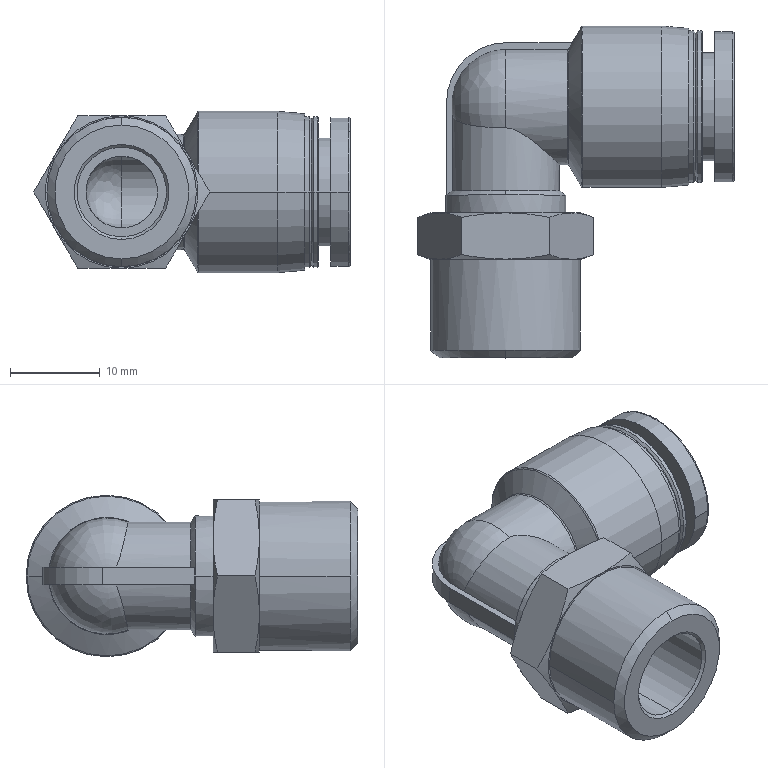Part | STEP file | L-type fitting PL1003 | 1 solid | 88 faces | box 35.315 x 37 x 18 mm | volume 6710 mm3 | cone 28 | cylinder 27 | plane 19 | spline 12 | other 2 | commonest cylinder face diameters 8 x4 10 x4 16.9 x4 13.4 x3 12 x2 12.1 x2